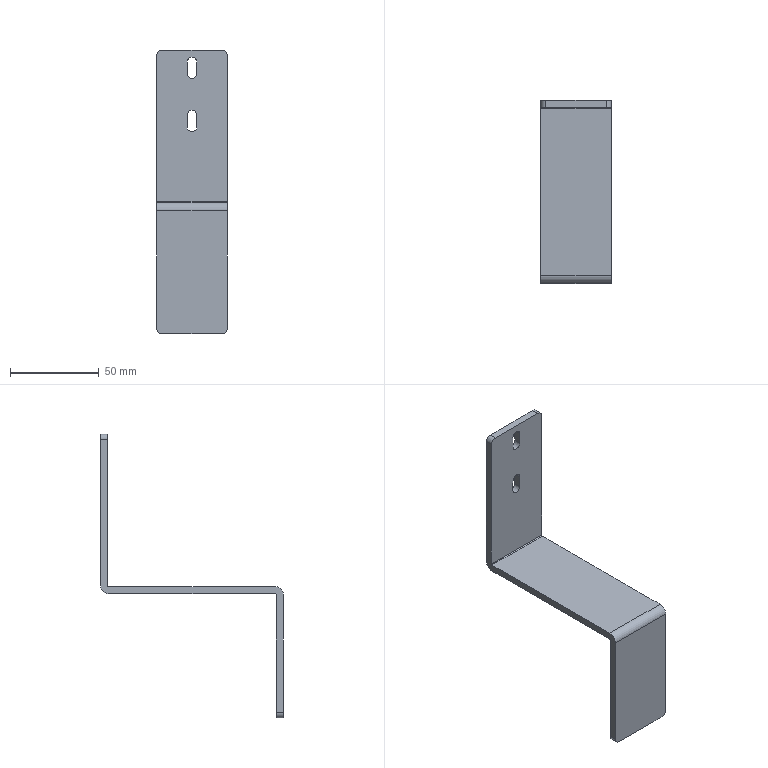Part | STEP file | HJDX-303 | 1 solid | 28 faces | box 40 x 103 x 160 mm | volume 40590 mm3 | cylinder 14 | plane 14 | commonest cylinder face diameters 5.5 x6 6 x4 1 x2 9 x2
STEP:
#1=CARTESIAN_POINT('',(2.75,-4.,-36.75));
#2=VERTEX_POINT('',#1);
#3=CARTESIAN_POINT('',(0.,-4.,-34.));
#4=VERTEX_POINT('',#3);
#5=CARTESIAN_POINT('',(0.,-4.,-36.75));
#6=DIRECTION('',(0.,-1.,0.));
#7=DIRECTION('',(0.,0.,1.));
#8=AXIS2_PLACEMENT_3D('',#5,#6,#7);
#9=CIRCLE('',#8,2.75);
#10=EDGE_CURVE('',#2,#4,#9,.T.);
#11=ORIENTED_EDGE('',*,*,#10,.T.);
#12=CARTESIAN_POINT('',(0.,0.,-34.));
#13=VERTEX_POINT('',#12);
#14=CARTESIAN_POINT('',(0.,0.,-34.));
#15=DIRECTION('',(0.,1.,0.));
#16=VECTOR('',#15,1000.);
#17=LINE('',#14,#16);
#18=EDGE_CURVE('',#4,#13,#17,.T.);
#19=ORIENTED_EDGE('',*,*,#18,.T.);
#20=CARTESIAN_POINT('',(2.75,0.,-36.75));
#21=VERTEX_POINT('',#20);
#22=CARTESIAN_POINT('',(0.,0.,-36.75));
#23=DIRECTION('',(0.,-1.,0.));
#24=DIRECTION('',(0.,0.,1.));
#25=AXIS2_PLACEMENT_3D('',#22,#23,#24);
#26=CIRCLE('',#25,2.75);
#27=EDGE_CURVE('',#21,#13,#26,.T.);
#28=ORIENTED_EDGE('',*,*,#27,.F.);
#29=CARTESIAN_POINT('',(2.75,-103.,-36.75));
#30=DIRECTION('',(0.,1.,0.));
#31=VECTOR('',#30,1000.);
#32=LINE('',#29,#31);
#33=EDGE_CURVE('',#2,#21,#32,.T.);
#34=ORIENTED_EDGE('',*,*,#33,.F.);
#35=EDGE_LOOP('',(#11,#19,#28,#34));
#36=FACE_OUTER_BOUND('',#35,.T.);
#37=CARTESIAN_POINT('',(0.,0.,-36.75));
#38=DIRECTION('',(0.,1.,0.));
#39=DIRECTION('',(0.,0.,1.));
#40=AXIS2_PLACEMENT_3D('',#37,#38,#39);
#41=CYLINDRICAL_SURFACE('',#40,2.75);
#42=ADVANCED_FACE('',(#36),#41,.F.);
#43=CARTESIAN_POINT('',(2.75,-4.,-6.75));
#44=VERTEX_POINT('',#43);
#45=CARTESIAN_POINT('',(0.,-4.,-4.));
#46=VERTEX_POINT('',#45);
#47=CARTESIAN_POINT('',(0.,-4.,-6.75));
#48=DIRECTION('',(0.,-1.,0.));
#49=DIRECTION('',(0.,0.,1.));
#50=AXIS2_PLACEMENT_3D('',#47,#48,#49);
#51=CIRCLE('',#50,2.75);
#52=EDGE_CURVE('',#44,#46,#51,.T.);
#53=ORIENTED_EDGE('',*,*,#52,.T.);
#54=CARTESIAN_POINT('',(0.,0.,-4.));
#55=VERTEX_POINT('',#54);
#56=CARTESIAN_POINT('',(0.,0.,-4.));
#57=DIRECTION('',(0.,1.,0.));
#58=VECTOR('',#57,1000.);
#59=LINE('',#56,#58);
#60=EDGE_CURVE('',#46,#55,#59,.T.);
#61=ORIENTED_EDGE('',*,*,#60,.T.);
#62=CARTESIAN_POINT('',(2.75,0.,-6.75));
#63=VERTEX_POINT('',#62);
#64=CARTESIAN_POINT('',(0.,0.,-6.75));
#65=DIRECTION('',(0.,-1.,0.));
#66=DIRECTION('',(0.,0.,1.));
#67=AXIS2_PLACEMENT_3D('',#64,#65,#66);
#68=CIRCLE('',#67,2.75);
#69=EDGE_CURVE('',#63,#55,#68,.T.);
#70=ORIENTED_EDGE('',*,*,#69,.F.);
#71=CARTESIAN_POINT('',(2.75,0.,-6.75));
#72=DIRECTION('',(0.,1.,0.));
#73=VECTOR('',#72,1000.);
#74=LINE('',#71,#73);
#75=EDGE_CURVE('',#44,#63,#74,.T.);
#76=ORIENTED_EDGE('',*,*,#75,.F.);
#77=EDGE_LOOP('',(#53,#61,#70,#76));
#78=FACE_OUTER_BOUND('',#77,.T.);
#79=CARTESIAN_POINT('',(0.,0.,-6.75));
#80=DIRECTION('',(0.,1.,0.));
#81=DIRECTION('',(0.,0.,1.));
#82=AXIS2_PLACEMENT_3D('',#79,#80,#81);
#83=CYLINDRICAL_SURFACE('',#82,2.75);
#84=ADVANCED_FACE('',(#78),#83,.F.);
#85=CARTESIAN_POINT('',(20.,-98.5,-86.));
#86=VERTEX_POINT('',#85);
#87=CARTESIAN_POINT('',(-20.,-98.5,-86.));
#88=VERTEX_POINT('',#87);
#89=CARTESIAN_POINT('',(20.,-98.5,-86.));
#90=DIRECTION('',(-1.,0.,0.));
#91=VECTOR('',#90,1000.);
#92=LINE('',#89,#91);
#93=EDGE_CURVE('',#86,#88,#92,.T.);
#94=ORIENTED_EDGE('',*,*,#93,.F.);
#95=CARTESIAN_POINT('',(20.,-4.5,-86.));
#96=VERTEX_POINT('',#95);
#97=CARTESIAN_POINT('',(20.,0.,-86.));
#98=DIRECTION('',(0.,-1.,0.));
#99=VECTOR('',#98,1000.);
#100=LINE('',#97,#99);
#101=EDGE_CURVE('',#96,#86,#100,.T.);
#102=ORIENTED_EDGE('',*,*,#101,.F.);
#103=CARTESIAN_POINT('',(-20.,-4.5,-86.));
#104=VERTEX_POINT('',#103);
#105=CARTESIAN_POINT('',(20.,-4.5,-86.));
#106=DIRECTION('',(1.,0.,0.));
#107=VECTOR('',#106,1000.);
#108=LINE('',#105,#107);
#109=EDGE_CURVE('',#104,#96,#108,.T.);
#110=ORIENTED_EDGE('',*,*,#109,.F.);
#111=CARTESIAN_POINT('',(-20.,0.,-86.));
#112=DIRECTION('',(0.,1.,0.));
#113=VECTOR('',#112,1000.);
#114=LINE('',#111,#113);
#115=EDGE_CURVE('',#88,#104,#114,.T.);
#116=ORIENTED_EDGE('',*,*,#115,.F.);
#117=EDGE_LOOP('',(#94,#102,#110,#116));
#118=FACE_OUTER_BOUND('',#117,.T.);
#119=CARTESIAN_POINT('',(20.,0.,-86.));
#120=DIRECTION('',(0.,0.,-1.));
#121=DIRECTION('',(0.,1.,0.));
#122=AXIS2_PLACEMENT_3D('',#119,#120,#121);
#123=PLANE('',#122);
#124=ADVANCED_FACE('',(#118),#123,.F.);
#125=ORIENTED_EDGE('',*,*,#115,.T.);
#126=CARTESIAN_POINT('',(-20.,-4.,-85.5));
#127=VERTEX_POINT('',#126);
#128=CARTESIAN_POINT('',(-20.,-4.5,-85.5));
#129=DIRECTION('',(1.,0.,0.));
#130=DIRECTION('',(0.,0.,1.));
#131=AXIS2_PLACEMENT_3D('',#128,#129,#130);
#132=CIRCLE('',#131,0.5);
#133=EDGE_CURVE('',#104,#127,#132,.T.);
#134=ORIENTED_EDGE('',*,*,#133,.T.);
#135=CARTESIAN_POINT('',(-20.,-4.,-3.));
#136=VERTEX_POINT('',#135);
#137=CARTESIAN_POINT('',(-20.,-4.,0.));
#138=DIRECTION('',(0.,0.,1.));
#139=VECTOR('',#138,1000.);
#140=LINE('',#137,#139);
#141=EDGE_CURVE('',#127,#136,#140,.T.);
#142=ORIENTED_EDGE('',*,*,#141,.T.);
#143=CARTESIAN_POINT('',(-20.,0.,-3.));
#144=VERTEX_POINT('',#143);
#145=CARTESIAN_POINT('',(-20.,-4.5,-3.));
#146=DIRECTION('',(0.,1.,0.));
#147=VECTOR('',#146,1000.);
#148=LINE('',#145,#147);
#149=EDGE_CURVE('',#136,#144,#148,.T.);
#150=ORIENTED_EDGE('',*,*,#149,.T.);
#151=CARTESIAN_POINT('',(-20.,0.,-85.5));
#152=VERTEX_POINT('',#151);
#153=CARTESIAN_POINT('',(-20.,0.,-86.));
#154=DIRECTION('',(0.,0.,-1.));
#155=VECTOR('',#154,1000.);
#156=LINE('',#153,#155);
#157=EDGE_CURVE('',#144,#152,#156,.T.);
#158=ORIENTED_EDGE('',*,*,#157,.T.);
#159=CARTESIAN_POINT('',(-20.,-4.5,-90.));
#160=VERTEX_POINT('',#159);
#161=CARTESIAN_POINT('',(-20.,-4.5,-85.5));
#162=DIRECTION('',(-1.,0.,0.));
#163=DIRECTION('',(0.,0.,1.));
#164=AXIS2_PLACEMENT_3D('',#161,#162,#163);
#165=CIRCLE('',#164,4.5);
#166=EDGE_CURVE('',#152,#160,#165,.T.);
#167=ORIENTED_EDGE('',*,*,#166,.T.);
#168=CARTESIAN_POINT('',(-20.,-98.5,-90.));
#169=VERTEX_POINT('',#168);
#170=CARTESIAN_POINT('',(-20.,-103.,-90.));
#171=DIRECTION('',(0.,-1.,0.));
#172=VECTOR('',#171,1000.);
#173=LINE('',#170,#172);
#174=EDGE_CURVE('',#160,#169,#173,.T.);
#175=ORIENTED_EDGE('',*,*,#174,.T.);
#176=CARTESIAN_POINT('',(-20.,-99.,-90.5));
#177=VERTEX_POINT('',#176);
#178=CARTESIAN_POINT('',(-20.,-98.5,-90.5));
#179=DIRECTION('',(1.,0.,0.));
#180=DIRECTION('',(0.,0.,1.));
#181=AXIS2_PLACEMENT_3D('',#178,#179,#180);
#182=CIRCLE('',#181,0.5);
#183=EDGE_CURVE('',#169,#177,#182,.T.);
#184=ORIENTED_EDGE('',*,*,#183,.T.);
#185=CARTESIAN_POINT('',(-20.,-99.,-157.));
#186=VERTEX_POINT('',#185);
#187=CARTESIAN_POINT('',(-20.,-99.,-90.5));
#188=DIRECTION('',(0.,0.,-1.));
#189=VECTOR('',#188,1000.);
#190=LINE('',#187,#189);
#191=EDGE_CURVE('',#177,#186,#190,.T.);
#192=ORIENTED_EDGE('',*,*,#191,.T.);
#193=CARTESIAN_POINT('',(-20.,-103.,-157.));
#194=VERTEX_POINT('',#193);
#195=CARTESIAN_POINT('',(-20.,-98.5,-157.));
#196=DIRECTION('',(0.,-1.,0.));
#197=VECTOR('',#196,1000.);
#198=LINE('',#195,#197);
#199=EDGE_CURVE('',#186,#194,#198,.T.);
#200=ORIENTED_EDGE('',*,*,#199,.T.);
#201=CARTESIAN_POINT('',(-20.,-103.,-90.5));
#202=VERTEX_POINT('',#201);
#203=CARTESIAN_POINT('',(-20.,-103.,-90.));
#204=DIRECTION('',(0.,0.,1.));
#205=VECTOR('',#204,1000.);
#206=LINE('',#203,#205);
#207=EDGE_CURVE('',#194,#202,#206,.T.);
#208=ORIENTED_EDGE('',*,*,#207,.T.);
#209=CARTESIAN_POINT('',(-20.,-98.5,-90.5));
#210=DIRECTION('',(1.,0.,0.));
#211=DIRECTION('',(0.,0.,1.));
#212=AXIS2_PLACEMENT_3D('',#209,#210,#211);
#213=CIRCLE('',#212,4.5);
#214=EDGE_CURVE('',#88,#202,#213,.T.);
#215=ORIENTED_EDGE('',*,*,#214,.F.);
#216=EDGE_LOOP('',(#125,#134,#142,#150,#158,#167,#175,#184,#192,#200,#208,#215));
#217=FACE_OUTER_BOUND('',#216,.T.);
#218=CARTESIAN_POINT('',(-20.,-103.,-90.5));
#219=DIRECTION('',(-1.,0.,0.));
#220=DIRECTION('',(0.,0.,1.));
#221=AXIS2_PLACEMENT_3D('',#218,#219,#220);
#222=PLANE('',#221);
#223=ADVANCED_FACE('',(#217),#222,.T.);
#224=CARTESIAN_POINT('',(20.,-103.,-90.5));
#225=VERTEX_POINT('',#224);
#226=CARTESIAN_POINT('',(20.,-98.5,-90.5));
#227=DIRECTION('',(-1.,0.,0.));
#228=DIRECTION('',(0.,0.,1.));
#229=AXIS2_PLACEMENT_3D('',#226,#227,#228);
#230=CIRCLE('',#229,4.5);
#231=EDGE_CURVE('',#225,#86,#230,.T.);
#232=ORIENTED_EDGE('',*,*,#231,.T.);
#233=ORIENTED_EDGE('',*,*,#93,.T.);
#234=ORIENTED_EDGE('',*,*,#214,.T.);
#235=CARTESIAN_POINT('',(20.,-103.,-90.5));
#236=DIRECTION('',(1.,0.,0.));
#237=VECTOR('',#236,1000.);
#238=LINE('',#235,#237);
#239=EDGE_CURVE('',#202,#225,#238,.T.);
#240=ORIENTED_EDGE('',*,*,#239,.T.);
#241=EDGE_LOOP('',(#232,#233,#234,#240));
#242=FACE_OUTER_BOUND('',#241,.T.);
#243=CARTESIAN_POINT('',(20.,-98.5,-90.5));
#244=DIRECTION('',(-1.,0.,0.));
#245=DIRECTION('',(0.,0.,1.));
#246=AXIS2_PLACEMENT_3D('',#243,#244,#245);
#247=CYLINDRICAL_SURFACE('',#246,4.5);
#248=ADVANCED_FACE('',(#242),#247,.T.);
#249=ORIENTED_EDGE('',*,*,#101,.T.);
#250=ORIENTED_EDGE('',*,*,#231,.F.);
#251=CARTESIAN_POINT('',(20.,-103.,-157.));
#252=VERTEX_POINT('',#251);
#253=CARTESIAN_POINT('',(20.,-103.,-90.));
#254=DIRECTION('',(0.,0.,-1.));
#255=VECTOR('',#254,1000.);
#256=LINE('',#253,#255);
#257=EDGE_CURVE('',#225,#252,#256,.T.);
#258=ORIENTED_EDGE('',*,*,#257,.T.);
#259=CARTESIAN_POINT('',(20.,-99.,-157.));
#260=VERTEX_POINT('',#259);
#261=CARTESIAN_POINT('',(20.,-98.5,-157.));
#262=DIRECTION('',(0.,1.,0.));
#263=VECTOR('',#262,1000.);
#264=LINE('',#261,#263);
#265=EDGE_CURVE('',#252,#260,#264,.T.);
#266=ORIENTED_EDGE('',*,*,#265,.T.);
#267=CARTESIAN_POINT('',(20.,-99.,-90.5));
#268=VERTEX_POINT('',#267);
#269=CARTESIAN_POINT('',(20.,-99.,-86.));
#270=DIRECTION('',(0.,0.,1.));
#271=VECTOR('',#270,1000.);
#272=LINE('',#269,#271);
#273=EDGE_CURVE('',#260,#268,#272,.T.);
#274=ORIENTED_EDGE('',*,*,#273,.T.);
#275=CARTESIAN_POINT('',(20.,-98.5,-90.));
#276=VERTEX_POINT('',#275);
#277=CARTESIAN_POINT('',(20.,-98.5,-90.5));
#278=DIRECTION('',(-1.,0.,0.));
#279=DIRECTION('',(0.,0.,1.));
#280=AXIS2_PLACEMENT_3D('',#277,#278,#279);
#281=CIRCLE('',#280,0.5);
#282=EDGE_CURVE('',#268,#276,#281,.T.);
#283=ORIENTED_EDGE('',*,*,#282,.T.);
#284=CARTESIAN_POINT('',(20.,-4.5,-90.));
#285=VERTEX_POINT('',#284);
#286=CARTESIAN_POINT('',(20.,-4.,-90.));
#287=DIRECTION('',(0.,1.,0.));
#288=VECTOR('',#287,1000.);
#289=LINE('',#286,#288);
#290=EDGE_CURVE('',#276,#285,#289,.T.);
#291=ORIENTED_EDGE('',*,*,#290,.T.);
#292=CARTESIAN_POINT('',(20.,0.,-85.5));
#293=VERTEX_POINT('',#292);
#294=CARTESIAN_POINT('',(20.,-4.5,-85.5));
#295=DIRECTION('',(1.,0.,0.));
#296=DIRECTION('',(0.,0.,1.));
#297=AXIS2_PLACEMENT_3D('',#294,#295,#296);
#298=CIRCLE('',#297,4.5);
#299=EDGE_CURVE('',#285,#293,#298,.T.);
#300=ORIENTED_EDGE('',*,*,#299,.T.);
#301=CARTESIAN_POINT('',(20.,0.,-3.));
#302=VERTEX_POINT('',#301);
#303=CARTESIAN_POINT('',(20.,0.,-90.5));
#304=DIRECTION('',(0.,0.,-1.));
#305=VECTOR('',#304,1000.);
#306=LINE('',#303,#305);
#307=EDGE_CURVE('',#302,#293,#306,.T.);
#308=ORIENTED_EDGE('',*,*,#307,.F.);
#309=CARTESIAN_POINT('',(20.,-4.,-3.));
#310=VERTEX_POINT('',#309);
#311=CARTESIAN_POINT('',(20.,-98.5,-3.));
#312=DIRECTION('',(0.,1.,0.));
#313=VECTOR('',#312,1000.);
#314=LINE('',#311,#313);
#315=EDGE_CURVE('',#310,#302,#314,.T.);
#316=ORIENTED_EDGE('',*,*,#315,.F.);
#317=CARTESIAN_POINT('',(20.,-4.,-85.5));
#318=VERTEX_POINT('',#317);
#319=CARTESIAN_POINT('',(20.,-4.,0.));
#320=DIRECTION('',(0.,0.,-1.));
#321=VECTOR('',#320,1000.);
#322=LINE('',#319,#321);
#323=EDGE_CURVE('',#310,#318,#322,.T.);
#324=ORIENTED_EDGE('',*,*,#323,.T.);
#325=CARTESIAN_POINT('',(20.,-4.5,-85.5));
#326=DIRECTION('',(-1.,0.,0.));
#327=DIRECTION('',(0.,0.,1.));
#328=AXIS2_PLACEMENT_3D('',#325,#326,#327);
#329=CIRCLE('',#328,0.5);
#330=EDGE_CURVE('',#318,#96,#329,.T.);
#331=ORIENTED_EDGE('',*,*,#330,.T.);
#332=EDGE_LOOP('',(#249,#250,#258,#266,#274,#283,#291,#300,#308,#316,#324,#331));
#333=FACE_OUTER_BOUND('',#332,.T.);
#334=CARTESIAN_POINT('',(20.,-4.,-85.5));
#335=DIRECTION('',(1.,0.,0.));
#336=DIRECTION('',(0.,0.,-1.));
#337=AXIS2_PLACEMENT_3D('',#334,#335,#336);
#338=PLANE('',#337);
#339=ADVANCED_FACE('',(#333),#338,.T.);
#340=ORIENTED_EDGE('',*,*,#109,.T.);
#341=ORIENTED_EDGE('',*,*,#330,.F.);
#342=CARTESIAN_POINT('',(20.,-4.,-85.5));
#343=DIRECTION('',(1.,0.,0.));
#344=VECTOR('',#343,1000.);
#345=LINE('',#342,#344);
#346=EDGE_CURVE('',#127,#318,#345,.T.);
#347=ORIENTED_EDGE('',*,*,#346,.F.);
#348=ORIENTED_EDGE('',*,*,#133,.F.);
#349=EDGE_LOOP('',(#340,#341,#347,#348));
#350=FACE_OUTER_BOUND('',#349,.T.);
#351=CARTESIAN_POINT('',(20.,-4.5,-85.5));
#352=DIRECTION('',(-1.,0.,0.));
#353=DIRECTION('',(0.,0.,1.));
#354=AXIS2_PLACEMENT_3D('',#351,#352,#353);
#355=CYLINDRICAL_SURFACE('',#354,0.5);
#356=ADVANCED_FACE('',(#350),#355,.F.);
#357=ORIENTED_EDGE('',*,*,#290,.F.);
#358=CARTESIAN_POINT('',(20.,-98.5,-90.));
#359=DIRECTION('',(-1.,0.,0.));
#360=VECTOR('',#359,1000.);
#361=LINE('',#358,#360);
#362=EDGE_CURVE('',#276,#169,#361,.T.);
#363=ORIENTED_EDGE('',*,*,#362,.T.);
#364=ORIENTED_EDGE('',*,*,#174,.F.);
#365=CARTESIAN_POINT('',(20.,-4.5,-90.));
#366=DIRECTION('',(1.,0.,0.));
#367=VECTOR('',#366,1000.);
#368=LINE('',#365,#367);
#369=EDGE_CURVE('',#160,#285,#368,.T.);
#370=ORIENTED_EDGE('',*,*,#369,.T.);
#371=EDGE_LOOP('',(#357,#363,#364,#370));
#372=FACE_OUTER_BOUND('',#371,.T.);
#373=CARTESIAN_POINT('',(20.,0.,-90.));
#374=DIRECTION('',(0.,0.,-1.));
#375=DIRECTION('',(0.,1.,0.));
#376=AXIS2_PLACEMENT_3D('',#373,#374,#375);
#377=PLANE('',#376);
#378=ADVANCED_FACE('',(#372),#377,.T.);
#379=CARTESIAN_POINT('',(-17.,-103.,-160.));
#380=VERTEX_POINT('',#379);
#381=CARTESIAN_POINT('',(-17.,-103.,-157.));
#382=DIRECTION('',(0.,1.,0.));
#383=DIRECTION('',(0.,0.,-1.));
#384=AXIS2_PLACEMENT_3D('',#381,#382,#383);
#385=CIRCLE('',#384,3.);
#386=EDGE_CURVE('',#380,#194,#385,.T.);
#387=ORIENTED_EDGE('',*,*,#386,.F.);
#388=CARTESIAN_POINT('',(17.,-103.,-160.));
#389=VERTEX_POINT('',#388);
#390=CARTESIAN_POINT('',(20.,-103.,-160.));
#391=DIRECTION('',(-1.,0.,0.));
#392=VECTOR('',#391,1000.);
#393=LINE('',#390,#392);
#394=EDGE_CURVE('',#389,#380,#393,.T.);
#395=ORIENTED_EDGE('',*,*,#394,.F.);
#396=CARTESIAN_POINT('',(17.,-103.,-157.));
#397=DIRECTION('',(0.,1.,0.));
#398=DIRECTION('',(0.,0.,-1.));
#399=AXIS2_PLACEMENT_3D('',#396,#397,#398);
#400=CIRCLE('',#399,3.);
#401=EDGE_CURVE('',#252,#389,#400,.T.);
#402=ORIENTED_EDGE('',*,*,#401,.F.);
#403=ORIENTED_EDGE('',*,*,#257,.F.);
#404=ORIENTED_EDGE('',*,*,#239,.F.);
#405=ORIENTED_EDGE('',*,*,#207,.F.);
#406=EDGE_LOOP('',(#387,#395,#402,#403,#404,#405));
#407=FACE_OUTER_BOUND('',#406,.T.);
#408=CARTESIAN_POINT('',(20.,-103.,-90.));
#409=DIRECTION('',(0.,1.,0.));
#410=DIRECTION('',(0.,0.,1.));
#411=AXIS2_PLACEMENT_3D('',#408,#409,#410);
#412=PLANE('',#411);
#413=ADVANCED_FACE('',(#407),#412,.F.);
#414=CARTESIAN_POINT('',(-17.,-4.,0.));
#415=VERTEX_POINT('',#414);
#416=CARTESIAN_POINT('',(-17.,-4.,-3.));
#417=DIRECTION('',(0.,1.,0.));
#418=DIRECTION('',(0.,0.,1.));
#419=AXIS2_PLACEMENT_3D('',#416,#417,#418);
#420=CIRCLE('',#419,3.);
#421=EDGE_CURVE('',#136,#415,#420,.T.);
#422=ORIENTED_EDGE('',*,*,#421,.F.);
#423=ORIENTED_EDGE('',*,*,#141,.F.);
#424=ORIENTED_EDGE('',*,*,#346,.T.);
#425=ORIENTED_EDGE('',*,*,#323,.F.);
#426=CARTESIAN_POINT('',(17.,-4.,0.));
#427=VERTEX_POINT('',#426);
#428=CARTESIAN_POINT('',(17.,-4.,-3.));
#429=DIRECTION('',(0.,1.,0.));
#430=DIRECTION('',(0.,0.,-1.));
#431=AXIS2_PLACEMENT_3D('',#428,#429,#430);
#432=CIRCLE('',#431,3.);
#433=EDGE_CURVE('',#427,#310,#432,.T.);
#434=ORIENTED_EDGE('',*,*,#433,.F.);
#435=CARTESIAN_POINT('',(20.,-4.,0.));
#436=DIRECTION('',(1.,0.,0.));
#437=VECTOR('',#436,1000.);
#438=LINE('',#435,#437);
#439=EDGE_CURVE('',#415,#427,#438,.T.);
#440=ORIENTED_EDGE('',*,*,#439,.F.);
#441=EDGE_LOOP('',(#422,#423,#424,#425,#434,#440));
#442=FACE_OUTER_BOUND('',#441,.T.);
#443=CARTESIAN_POINT('',(-2.75,-4.,-43.25));
#444=VERTEX_POINT('',#443);
#445=CARTESIAN_POINT('',(2.75,-4.,-43.25));
#446=VERTEX_POINT('',#445);
#447=CARTESIAN_POINT('',(0.,-4.,-43.25));
#448=DIRECTION('',(0.,-1.,0.));
#449=DIRECTION('',(0.,0.,1.));
#450=AXIS2_PLACEMENT_3D('',#447,#448,#449);
#451=CIRCLE('',#450,2.75);
#452=EDGE_CURVE('',#444,#446,#451,.T.);
#453=ORIENTED_EDGE('',*,*,#452,.F.);
#454=CARTESIAN_POINT('',(-2.75,-4.,-36.75));
#455=VERTEX_POINT('',#454);
#456=CARTESIAN_POINT('',(-2.75,-4.,0.));
#457=DIRECTION('',(0.,0.,-1.));
#458=VECTOR('',#457,1000.);
#459=LINE('',#456,#458);
#460=EDGE_CURVE('',#455,#444,#459,.T.);
#461=ORIENTED_EDGE('',*,*,#460,.F.);
#462=CARTESIAN_POINT('',(0.,-4.,-36.75));
#463=DIRECTION('',(0.,-1.,0.));
#464=DIRECTION('',(0.,0.,1.));
#465=AXIS2_PLACEMENT_3D('',#462,#463,#464);
#466=CIRCLE('',#465,2.75);
#467=EDGE_CURVE('',#4,#455,#466,.T.);
#468=ORIENTED_EDGE('',*,*,#467,.F.);
#469=ORIENTED_EDGE('',*,*,#10,.F.);
#470=CARTESIAN_POINT('',(2.75,-4.,0.));
#471=DIRECTION('',(0.,0.,1.));
#472=VECTOR('',#471,1000.);
#473=LINE('',#470,#472);
#474=EDGE_CURVE('',#446,#2,#473,.T.);
#475=ORIENTED_EDGE('',*,*,#474,.F.);
#476=EDGE_LOOP('',(#453,#461,#468,#469,#475));
#477=FACE_BOUND('',#476,.T.);
#478=ORIENTED_EDGE('',*,*,#52,.F.);
#479=CARTESIAN_POINT('',(2.75,-4.,-13.25));
#480=VERTEX_POINT('',#479);
#481=CARTESIAN_POINT('',(2.75,-4.,0.));
#482=DIRECTION('',(0.,0.,1.));
#483=VECTOR('',#482,1000.);
#484=LINE('',#481,#483);
#485=EDGE_CURVE('',#480,#44,#484,.T.);
#486=ORIENTED_EDGE('',*,*,#485,.F.);
#487=CARTESIAN_POINT('',(-2.75,-4.,-13.25));
#488=VERTEX_POINT('',#487);
#489=CARTESIAN_POINT('',(0.,-4.,-13.25));
#490=DIRECTION('',(0.,-1.,0.));
#491=DIRECTION('',(0.,0.,1.));
#492=AXIS2_PLACEMENT_3D('',#489,#490,#491);
#493=CIRCLE('',#492,2.75);
#494=EDGE_CURVE('',#488,#480,#493,.T.);
#495=ORIENTED_EDGE('',*,*,#494,.F.);
#496=CARTESIAN_POINT('',(-2.75,-4.,-6.75));
#497=VERTEX_POINT('',#496);
#498=CARTESIAN_POINT('',(-2.75,-4.,0.));
#499=DIRECTION('',(0.,0.,-1.));
#500=VECTOR('',#499,1000.);
#501=LINE('',#498,#500);
#502=EDGE_CURVE('',#497,#488,#501,.T.);
#503=ORIENTED_EDGE('',*,*,#502,.F.);
#504=CARTESIAN_POINT('',(0.,-4.,-6.75));
#505=DIRECTION('',(0.,-1.,0.));
#506=DIRECTION('',(0.,0.,1.));
#507=AXIS2_PLACEMENT_3D('',#504,#505,#506);
#508=CIRCLE('',#507,2.75);
#509=EDGE_CURVE('',#46,#497,#508,.T.);
#510=ORIENTED_EDGE('',*,*,#509,.F.);
#511=EDGE_LOOP('',(#478,#486,#495,#503,#510));
#512=FACE_BOUND('',#511,.T.);
#513=CARTESIAN_POINT('',(20.,-4.,0.));
#514=DIRECTION('',(0.,1.,0.));
#515=DIRECTION('',(0.,0.,1.));
#516=AXIS2_PLACEMENT_3D('',#513,#514,#515);
#517=PLANE('',#516);
#518=ADVANCED_FACE('',(#442,#477,#512),#517,.F.);
#519=ORIENTED_EDGE('',*,*,#299,.F.);
#520=ORIENTED_EDGE('',*,*,#369,.F.);
#521=ORIENTED_EDGE('',*,*,#166,.F.);
#522=CARTESIAN_POINT('',(20.,0.,-85.5));
#523=DIRECTION('',(1.,0.,0.));
#524=VECTOR('',#523,1000.);
#525=LINE('',#522,#524);
#526=EDGE_CURVE('',#152,#293,#525,.T.);
#527=ORIENTED_EDGE('',*,*,#526,.T.);
#528=EDGE_LOOP('',(#519,#520,#521,#527));
#529=FACE_OUTER_BOUND('',#528,.T.);
#530=CARTESIAN_POINT('',(20.,-4.5,-85.5));
#531=DIRECTION('',(-1.,0.,0.));
#532=DIRECTION('',(0.,0.,1.));
#533=AXIS2_PLACEMENT_3D('',#530,#531,#532);
#534=CYLINDRICAL_SURFACE('',#533,4.5);
#535=ADVANCED_FACE('',(#529),#534,.T.);
#536=ORIENTED_EDGE('',*,*,#362,.F.);
#537=ORIENTED_EDGE('',*,*,#282,.F.);
#538=CARTESIAN_POINT('',(20.,-99.,-90.5));
#539=DIRECTION('',(1.,0.,0.));
#540=VECTOR('',#539,1000.);
#541=LINE('',#538,#540);
#542=EDGE_CURVE('',#177,#268,#541,.T.);
#543=ORIENTED_EDGE('',*,*,#542,.F.);
#544=ORIENTED_EDGE('',*,*,#183,.F.);
#545=EDGE_LOOP('',(#536,#537,#543,#544));
#546=FACE_OUTER_BOUND('',#545,.T.);
#547=CARTESIAN_POINT('',(20.,-98.5,-90.5));
#548=DIRECTION('',(-1.,0.,0.));
#549=DIRECTION('',(0.,0.,1.));
#550=AXIS2_PLACEMENT_3D('',#547,#548,#549);
#551=CYLINDRICAL_SURFACE('',#550,0.5);
#552=ADVANCED_FACE('',(#546),#551,.F.);
#553=ORIENTED_EDGE('',*,*,#386,.T.);
#554=ORIENTED_EDGE('',*,*,#199,.F.);
#555=CARTESIAN_POINT('',(-17.,-99.,-160.));
#556=VERTEX_POINT('',#555);
#557=CARTESIAN_POINT('',(-17.,-99.,-157.));
#558=DIRECTION('',(0.,-1.,0.));
#559=DIRECTION('',(0.,0.,-1.));
#560=AXIS2_PLACEMENT_3D('',#557,#558,#559);
#561=CIRCLE('',#560,3.);
#562=EDGE_CURVE('',#186,#556,#561,.T.);
#563=ORIENTED_EDGE('',*,*,#562,.T.);
#564=CARTESIAN_POINT('',(-17.,-98.5,-160.));
#565=DIRECTION('',(0.,-1.,0.));
#566=VECTOR('',#565,1000.);
#567=LINE('',#564,#566);
#568=EDGE_CURVE('',#556,#380,#567,.T.);
#569=ORIENTED_EDGE('',*,*,#568,.T.);
#570=EDGE_LOOP('',(#553,#554,#563,#569));
#571=FACE_OUTER_BOUND('',#570,.T.);
#572=CARTESIAN_POINT('',(-17.,-98.5,-157.));
#573=DIRECTION('',(0.,-1.,0.));
#574=DIRECTION('',(0.,0.,-1.));
#575=AXIS2_PLACEMENT_3D('',#572,#573,#574);
#576=CYLINDRICAL_SURFACE('',#575,3.);
#577=ADVANCED_FACE('',(#571),#576,.T.);
#578=CARTESIAN_POINT('',(17.,-99.,-160.));
#579=VERTEX_POINT('',#578);
#580=CARTESIAN_POINT('',(20.,-99.,-160.));
#581=DIRECTION('',(1.,0.,0.));
#582=VECTOR('',#581,1000.);
#583=LINE('',#580,#582);
#584=EDGE_CURVE('',#556,#579,#583,.T.);
#585=ORIENTED_EDGE('',*,*,#584,.T.);
#586=CARTESIAN_POINT('',(17.,-99.,-160.));
#587=DIRECTION('',(0.,-1.,0.));
#588=VECTOR('',#587,1000.);
#589=LINE('',#586,#588);
#590=EDGE_CURVE('',#579,#389,#589,.T.);
#591=ORIENTED_EDGE('',*,*,#590,.T.);
#592=ORIENTED_EDGE('',*,*,#394,.T.);
#593=ORIENTED_EDGE('',*,*,#568,.F.);
#594=EDGE_LOOP('',(#585,#591,#592,#593));
#595=FACE_OUTER_BOUND('',#594,.T.);
#596=CARTESIAN_POINT('',(20.,-99.,-160.));
#597=DIRECTION('',(0.,0.,-1.));
#598=DIRECTION('',(-1.,0.,0.));
#599=AXIS2_PLACEMENT_3D('',#596,#597,#598);
#600=PLANE('',#599);
#601=ADVANCED_FACE('',(#595),#600,.T.);
#602=ORIENTED_EDGE('',*,*,#401,.T.);
#603=ORIENTED_EDGE('',*,*,#590,.F.);
#604=CARTESIAN_POINT('',(17.,-99.,-157.));
#605=DIRECTION('',(0.,-1.,0.));
#606=DIRECTION('',(0.,0.,-1.));
#607=AXIS2_PLACEMENT_3D('',#604,#605,#606);
#608=CIRCLE('',#607,3.);
#609=EDGE_CURVE('',#579,#260,#608,.T.);
#610=ORIENTED_EDGE('',*,*,#609,.T.);
#611=ORIENTED_EDGE('',*,*,#265,.F.);
#612=EDGE_LOOP('',(#602,#603,#610,#611));
#613=FACE_OUTER_BOUND('',#612,.T.);
#614=CARTESIAN_POINT('',(17.,-99.,-157.));
#615=DIRECTION('',(0.,-1.,0.));
#616=DIRECTION('',(0.,0.,-1.));
#617=AXIS2_PLACEMENT_3D('',#614,#615,#616);
#618=CYLINDRICAL_SURFACE('',#617,3.);
#619=ADVANCED_FACE('',(#613),#618,.T.);
#620=ORIENTED_EDGE('',*,*,#439,.T.);
#621=CARTESIAN_POINT('',(17.,0.,0.));
#622=VERTEX_POINT('',#621);
#623=CARTESIAN_POINT('',(17.,-4.,0.));
#624=DIRECTION('',(0.,1.,0.));
#625=VECTOR('',#624,1000.);
#626=LINE('',#623,#625);
#627=EDGE_CURVE('',#427,#622,#626,.T.);
#628=ORIENTED_EDGE('',*,*,#627,.T.);
#629=CARTESIAN_POINT('',(-17.,0.,0.));
#630=VERTEX_POINT('',#629);
#631=CARTESIAN_POINT('',(20.,0.,0.));
#632=DIRECTION('',(-1.,0.,0.));
#633=VECTOR('',#632,1000.);
#634=LINE('',#631,#633);
#635=EDGE_CURVE('',#622,#630,#634,.T.);
#636=ORIENTED_EDGE('',*,*,#635,.T.);
#637=CARTESIAN_POINT('',(-17.,-4.,0.));
#638=DIRECTION('',(0.,-1.,0.));
#639=VECTOR('',#638,1000.);
#640=LINE('',#637,#639);
#641=EDGE_CURVE('',#630,#415,#640,.T.);
#642=ORIENTED_EDGE('',*,*,#641,.T.);
#643=EDGE_LOOP('',(#620,#628,#636,#642));
#644=FACE_OUTER_BOUND('',#643,.T.);
#645=CARTESIAN_POINT('',(20.,-4.,0.));
#646=DIRECTION('',(0.,0.,1.));
#647=DIRECTION('',(1.,0.,0.));
#648=AXIS2_PLACEMENT_3D('',#645,#646,#647);
#649=PLANE('',#648);
#650=ADVANCED_FACE('',(#644),#649,.T.);
#651=CARTESIAN_POINT('',(-17.,0.,-3.));
#652=DIRECTION('',(0.,-1.,0.));
#653=DIRECTION('',(0.,0.,1.));
#654=AXIS2_PLACEMENT_3D('',#651,#652,#653);
#655=CIRCLE('',#654,3.);
#656=EDGE_CURVE('',#630,#144,#655,.T.);
#657=ORIENTED_EDGE('',*,*,#656,.T.);
#658=ORIENTED_EDGE('',*,*,#149,.F.);
#659=ORIENTED_EDGE('',*,*,#421,.T.);
#660=ORIENTED_EDGE('',*,*,#641,.F.);
#661=EDGE_LOOP('',(#657,#658,#659,#660));
#662=FACE_OUTER_BOUND('',#661,.T.);
#663=CARTESIAN_POINT('',(-17.,-4.5,-3.));
#664=DIRECTION('',(0.,1.,0.));
#665=DIRECTION('',(0.,0.,1.));
#666=AXIS2_PLACEMENT_3D('',#663,#664,#665);
#667=CYLINDRICAL_SURFACE('',#666,3.);
#668=ADVANCED_FACE('',(#662),#667,.T.);
#669=CARTESIAN_POINT('',(17.,0.,-3.));
#670=DIRECTION('',(0.,-1.,0.));
#671=DIRECTION('',(0.,0.,-1.));
#672=AXIS2_PLACEMENT_3D('',#669,#670,#671);
#673=CIRCLE('',#672,3.);
#674=EDGE_CURVE('',#302,#622,#673,.T.);
#675=ORIENTED_EDGE('',*,*,#674,.T.);
#676=ORIENTED_EDGE('',*,*,#627,.F.);
#677=ORIENTED_EDGE('',*,*,#433,.T.);
#678=ORIENTED_EDGE('',*,*,#315,.T.);
#679=EDGE_LOOP('',(#675,#676,#677,#678));
#680=FACE_OUTER_BOUND('',#679,.T.);
#681=CARTESIAN_POINT('',(17.,-4.,-3.));
#682=DIRECTION('',(0.,-1.,0.));
#683=DIRECTION('',(0.,0.,-1.));
#684=AXIS2_PLACEMENT_3D('',#681,#682,#683);
#685=CYLINDRICAL_SURFACE('',#684,3.);
#686=ADVANCED_FACE('',(#680),#685,.T.);
#687=CARTESIAN_POINT('',(2.75,0.,-43.25));
#688=VERTEX_POINT('',#687);
#689=CARTESIAN_POINT('',(2.75,0.,-43.25));
#690=DIRECTION('',(0.,0.,-1.));
#691=VECTOR('',#690,1000.);
#692=LINE('',#689,#691);
#693=EDGE_CURVE('',#21,#688,#692,.T.);
#694=ORIENTED_EDGE('',*,*,#693,.T.);
#695=CARTESIAN_POINT('',(2.75,-103.,-43.25));
#696=DIRECTION('',(0.,-1.,0.));
#697=VECTOR('',#696,1000.);
#698=LINE('',#695,#697);
#699=EDGE_CURVE('',#688,#446,#698,.T.);
#700=ORIENTED_EDGE('',*,*,#699,.T.);
#701=ORIENTED_EDGE('',*,*,#474,.T.);
#702=ORIENTED_EDGE('',*,*,#33,.T.);
#703=EDGE_LOOP('',(#694,#700,#701,#702));
#704=FACE_OUTER_BOUND('',#703,.T.);
#705=CARTESIAN_POINT('',(2.75,-103.,-43.25));
#706=DIRECTION('',(-1.,0.,0.));
#707=DIRECTION('',(0.,0.,1.));
#708=AXIS2_PLACEMENT_3D('',#705,#706,#707);
#709=PLANE('',#708);
#710=ADVANCED_FACE('',(#704),#709,.T.);
#711=CARTESIAN_POINT('',(-2.75,0.,-43.25));
#712=VERTEX_POINT('',#711);
#713=CARTESIAN_POINT('',(0.,0.,-43.25));
#714=DIRECTION('',(0.,-1.,0.));
#715=DIRECTION('',(0.,0.,1.));
#716=AXIS2_PLACEMENT_3D('',#713,#714,#715);
#717=CIRCLE('',#716,2.75);
#718=EDGE_CURVE('',#712,#688,#717,.T.);
#719=ORIENTED_EDGE('',*,*,#718,.F.);
#720=CARTESIAN_POINT('',(-2.75,0.,-43.25));
#721=DIRECTION('',(0.,1.,0.));
#722=VECTOR('',#721,1000.);
#723=LINE('',#720,#722);
#724=EDGE_CURVE('',#444,#712,#723,.T.);
#725=ORIENTED_EDGE('',*,*,#724,.F.);
#726=ORIENTED_EDGE('',*,*,#452,.T.);
#727=ORIENTED_EDGE('',*,*,#699,.F.);
#728=EDGE_LOOP('',(#719,#725,#726,#727));
#729=FACE_OUTER_BOUND('',#728,.T.);
#730=CARTESIAN_POINT('',(0.,0.,-43.25));
#731=DIRECTION('',(0.,1.,0.));
#732=DIRECTION('',(0.,0.,1.));
#733=AXIS2_PLACEMENT_3D('',#730,#731,#732);
#734=CYLINDRICAL_SURFACE('',#733,2.75);
#735=ADVANCED_FACE('',(#729),#734,.F.);
#736=CARTESIAN_POINT('',(-2.75,0.,-36.75));
#737=VERTEX_POINT('',#736);
#738=CARTESIAN_POINT('',(-2.75,0.,-43.25));
#739=DIRECTION('',(0.,0.,-1.));
#740=VECTOR('',#739,1000.);
#741=LINE('',#738,#740);
#742=EDGE_CURVE('',#737,#712,#741,.T.);
#743=ORIENTED_EDGE('',*,*,#742,.F.);
#744=CARTESIAN_POINT('',(-2.75,0.,-36.75));
#745=DIRECTION('',(0.,1.,0.));
#746=VECTOR('',#745,1000.);
#747=LINE('',#744,#746);
#748=EDGE_CURVE('',#455,#737,#747,.T.);
#749=ORIENTED_EDGE('',*,*,#748,.F.);
#750=ORIENTED_EDGE('',*,*,#460,.T.);
#751=ORIENTED_EDGE('',*,*,#724,.T.);
#752=EDGE_LOOP('',(#743,#749,#750,#751));
#753=FACE_OUTER_BOUND('',#752,.T.);
#754=CARTESIAN_POINT('',(-2.75,0.,-43.25));
#755=DIRECTION('',(-1.,0.,0.));
#756=DIRECTION('',(0.,0.,1.));
#757=AXIS2_PLACEMENT_3D('',#754,#755,#756);
#758=PLANE('',#757);
#759=ADVANCED_FACE('',(#753),#758,.F.);
#760=ORIENTED_EDGE('',*,*,#18,.F.);
#761=ORIENTED_EDGE('',*,*,#467,.T.);
#762=ORIENTED_EDGE('',*,*,#748,.T.);
#763=CARTESIAN_POINT('',(0.,0.,-36.75));
#764=DIRECTION('',(0.,-1.,0.));
#765=DIRECTION('',(0.,0.,1.));
#766=AXIS2_PLACEMENT_3D('',#763,#764,#765);
#767=CIRCLE('',#766,2.75);
#768=EDGE_CURVE('',#13,#737,#767,.T.);
#769=ORIENTED_EDGE('',*,*,#768,.F.);
#770=EDGE_LOOP('',(#760,#761,#762,#769));
#771=FACE_OUTER_BOUND('',#770,.T.);
#772=CARTESIAN_POINT('',(0.,0.,-36.75));
#773=DIRECTION('',(0.,1.,0.));
#774=DIRECTION('',(0.,0.,1.));
#775=AXIS2_PLACEMENT_3D('',#772,#773,#774);
#776=CYLINDRICAL_SURFACE('',#775,2.75);
#777=ADVANCED_FACE('',(#771),#776,.F.);
#778=CARTESIAN_POINT('',(-2.75,0.,-6.75));
#779=VERTEX_POINT('',#778);
#780=CARTESIAN_POINT('',(-2.75,0.,-13.25));
#781=VERTEX_POINT('',#780);
#782=CARTESIAN_POINT('',(-2.75,0.,-13.25));
#783=DIRECTION('',(0.,0.,-1.));
#784=VECTOR('',#783,1000.);
#785=LINE('',#782,#784);
#786=EDGE_CURVE('',#779,#781,#785,.T.);
#787=ORIENTED_EDGE('',*,*,#786,.F.);
#788=CARTESIAN_POINT('',(-2.75,0.,-6.75));
#789=DIRECTION('',(0.,1.,0.));
#790=VECTOR('',#789,1000.);
#791=LINE('',#788,#790);
#792=EDGE_CURVE('',#497,#779,#791,.T.);
#793=ORIENTED_EDGE('',*,*,#792,.F.);
#794=ORIENTED_EDGE('',*,*,#502,.T.);
#795=CARTESIAN_POINT('',(-2.75,0.,-13.25));
#796=DIRECTION('',(0.,-1.,0.));
#797=VECTOR('',#796,1000.);
#798=LINE('',#795,#797);
#799=EDGE_CURVE('',#781,#488,#798,.T.);
#800=ORIENTED_EDGE('',*,*,#799,.F.);
#801=EDGE_LOOP('',(#787,#793,#794,#800));
#802=FACE_OUTER_BOUND('',#801,.T.);
#803=CARTESIAN_POINT('',(-2.75,0.,-13.25));
#804=DIRECTION('',(-1.,0.,0.));
#805=DIRECTION('',(0.,0.,1.));
#806=AXIS2_PLACEMENT_3D('',#803,#804,#805);
#807=PLANE('',#806);
#808=ADVANCED_FACE('',(#802),#807,.F.);
#809=ORIENTED_EDGE('',*,*,#60,.F.);
#810=ORIENTED_EDGE('',*,*,#509,.T.);
#811=ORIENTED_EDGE('',*,*,#792,.T.);
#812=CARTESIAN_POINT('',(0.,0.,-6.75));
#813=DIRECTION('',(0.,-1.,0.));
#814=DIRECTION('',(0.,0.,1.));
#815=AXIS2_PLACEMENT_3D('',#812,#813,#814);
#816=CIRCLE('',#815,2.75);
#817=EDGE_CURVE('',#55,#779,#816,.T.);
#818=ORIENTED_EDGE('',*,*,#817,.F.);
#819=EDGE_LOOP('',(#809,#810,#811,#818));
#820=FACE_OUTER_BOUND('',#819,.T.);
#821=CARTESIAN_POINT('',(0.,0.,-6.75));
#822=DIRECTION('',(0.,1.,0.));
#823=DIRECTION('',(0.,0.,1.));
#824=AXIS2_PLACEMENT_3D('',#821,#822,#823);
#825=CYLINDRICAL_SURFACE('',#824,2.75);
#826=ADVANCED_FACE('',(#820),#825,.F.);
#827=CARTESIAN_POINT('',(2.75,0.,-13.25));
#828=VERTEX_POINT('',#827);
#829=CARTESIAN_POINT('',(2.75,0.,-13.25));
#830=DIRECTION('',(0.,0.,-1.));
#831=VECTOR('',#830,1000.);
#832=LINE('',#829,#831);
#833=EDGE_CURVE('',#63,#828,#832,.T.);
#834=ORIENTED_EDGE('',*,*,#833,.T.);
#835=CARTESIAN_POINT('',(2.75,-103.,-13.25));
#836=DIRECTION('',(0.,-1.,0.));
#837=VECTOR('',#836,1000.);
#838=LINE('',#835,#837);
#839=EDGE_CURVE('',#828,#480,#838,.T.);
#840=ORIENTED_EDGE('',*,*,#839,.T.);
#841=ORIENTED_EDGE('',*,*,#485,.T.);
#842=ORIENTED_EDGE('',*,*,#75,.T.);
#843=EDGE_LOOP('',(#834,#840,#841,#842));
#844=FACE_OUTER_BOUND('',#843,.T.);
#845=CARTESIAN_POINT('',(2.75,-103.,-13.25));
#846=DIRECTION('',(-1.,0.,0.));
#847=DIRECTION('',(0.,0.,1.));
#848=AXIS2_PLACEMENT_3D('',#845,#846,#847);
#849=PLANE('',#848);
#850=ADVANCED_FACE('',(#844),#849,.T.);
#851=CARTESIAN_POINT('',(0.,0.,-13.25));
#852=DIRECTION('',(0.,-1.,0.));
#853=DIRECTION('',(0.,0.,1.));
#854=AXIS2_PLACEMENT_3D('',#851,#852,#853);
#855=CIRCLE('',#854,2.75);
#856=EDGE_CURVE('',#781,#828,#855,.T.);
#857=ORIENTED_EDGE('',*,*,#856,.F.);
#858=ORIENTED_EDGE('',*,*,#799,.T.);
#859=ORIENTED_EDGE('',*,*,#494,.T.);
#860=ORIENTED_EDGE('',*,*,#839,.F.);
#861=EDGE_LOOP('',(#857,#858,#859,#860));
#862=FACE_OUTER_BOUND('',#861,.T.);
#863=CARTESIAN_POINT('',(0.,0.,-13.25));
#864=DIRECTION('',(0.,1.,0.));
#865=DIRECTION('',(0.,0.,1.));
#866=AXIS2_PLACEMENT_3D('',#863,#864,#865);
#867=CYLINDRICAL_SURFACE('',#866,2.75);
#868=ADVANCED_FACE('',(#862),#867,.F.);
#869=ORIENTED_EDGE('',*,*,#307,.T.);
#870=ORIENTED_EDGE('',*,*,#526,.F.);
#871=ORIENTED_EDGE('',*,*,#157,.F.);
#872=ORIENTED_EDGE('',*,*,#656,.F.);
#873=ORIENTED_EDGE('',*,*,#635,.F.);
#874=ORIENTED_EDGE('',*,*,#674,.F.);
#875=EDGE_LOOP('',(#869,#870,#871,#872,#873,#874));
#876=FACE_OUTER_BOUND('',#875,.T.);
#877=ORIENTED_EDGE('',*,*,#693,.F.);
#878=ORIENTED_EDGE('',*,*,#27,.T.);
#879=ORIENTED_EDGE('',*,*,#768,.T.);
#880=ORIENTED_EDGE('',*,*,#742,.T.);
#881=ORIENTED_EDGE('',*,*,#718,.T.);
#882=EDGE_LOOP('',(#877,#878,#879,#880,#881));
#883=FACE_BOUND('',#882,.T.);
#884=ORIENTED_EDGE('',*,*,#833,.F.);
#885=ORIENTED_EDGE('',*,*,#69,.T.);
#886=ORIENTED_EDGE('',*,*,#817,.T.);
#887=ORIENTED_EDGE('',*,*,#786,.T.);
#888=ORIENTED_EDGE('',*,*,#856,.T.);
#889=EDGE_LOOP('',(#884,#885,#886,#887,#888));
#890=FACE_BOUND('',#889,.T.);
#891=CARTESIAN_POINT('',(20.,0.,0.));
#892=DIRECTION('',(0.,1.,0.));
#893=DIRECTION('',(0.,0.,1.));
#894=AXIS2_PLACEMENT_3D('',#891,#892,#893);
#895=PLANE('',#894);
#896=ADVANCED_FACE('',(#876,#883,#890),#895,.T.);
#897=ORIENTED_EDGE('',*,*,#273,.F.);
#898=ORIENTED_EDGE('',*,*,#609,.F.);
#899=ORIENTED_EDGE('',*,*,#584,.F.);
#900=ORIENTED_EDGE('',*,*,#562,.F.);
#901=ORIENTED_EDGE('',*,*,#191,.F.);
#902=ORIENTED_EDGE('',*,*,#542,.T.);
#903=EDGE_LOOP('',(#897,#898,#899,#900,#901,#902));
#904=FACE_OUTER_BOUND('',#903,.T.);
#905=CARTESIAN_POINT('',(20.,-99.,-90.));
#906=DIRECTION('',(0.,1.,0.));
#907=DIRECTION('',(0.,0.,1.));
#908=AXIS2_PLACEMENT_3D('',#905,#906,#907);
#909=PLANE('',#908);
#910=ADVANCED_FACE('',(#904),#909,.T.);
#911=CLOSED_SHELL('',(#42,#84,#124,#223,#248,#339,#356,#378,#413,#518,#535,#552,#577,#601,#619,#650,#668,#686,#710,#735,#759,#777,#808,#826,#850,#868,#896,#910));
#912=MANIFOLD_SOLID_BREP('',#911);
#913=CARTESIAN_POINT('',(0.,0.,0.));
#914=DIRECTION('',(0.,0.,1.));
#915=DIRECTION('',(1.,0.,0.));
#916=AXIS2_PLACEMENT_3D('',#913,#914,#915);
#917=(LENGTH_UNIT()NAMED_UNIT(*)SI_UNIT(.MILLI.,.METRE.));
#918=UNCERTAINTY_MEASURE_WITH_UNIT(LENGTH_MEASURE(0.00001),#917,'','');
#919=(NAMED_UNIT(*)PLANE_ANGLE_UNIT()SI_UNIT($,.RADIAN.));
#920=(NAMED_UNIT(*)SI_UNIT($,.STERADIAN.)SOLID_ANGLE_UNIT());
#921=(GEOMETRIC_REPRESENTATION_CONTEXT(3)GLOBAL_UNCERTAINTY_ASSIGNED_CONTEXT((#918))GLOBAL_UNIT_ASSIGNED_CONTEXT((#917,#919,#920))REPRESENTATION_CONTEXT('',''));
#922=ADVANCED_BREP_SHAPE_REPRESENTATION('',(#912,#916),#921);